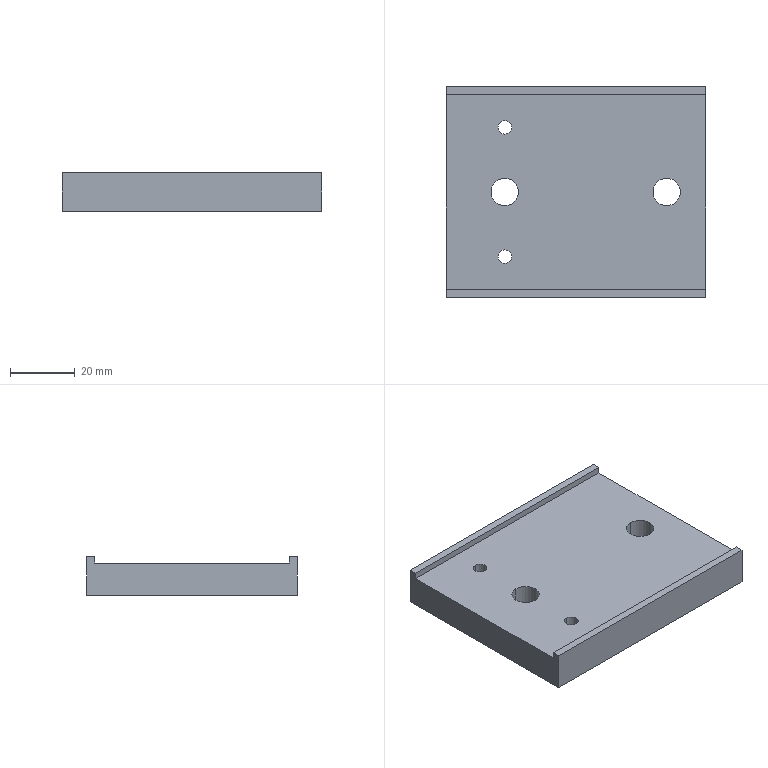Part | NX | 1 solid | 26 faces | box 80 x 65 x 12 mm | volume 50779 mm3 | cylinder 12 | plane 10 | cone 4 | commonest cylinder face diameters 4.2 x4 5 x4 8.5 x4
STEP:
#1=CARTESIAN_POINT('',(-22.,-17.9,-12.));
#2=VERTEX_POINT('',#1);
#3=CARTESIAN_POINT('',(-22.,-22.1,-12.));
#4=VERTEX_POINT('',#3);
#5=CARTESIAN_POINT('',(-22.,-20.,-12.));
#6=DIRECTION('',(0.,0.,1.));
#7=DIRECTION('',(0.,-1.,0.));
#8=AXIS2_PLACEMENT_3D('',#5,#6,#7);
#9=CIRCLE('',#8,2.1);
#10=EDGE_CURVE('',#2,#4,#9,.T.);
#11=ORIENTED_EDGE('',*,*,#10,.F.);
#12=CARTESIAN_POINT('',(-22.,-17.9,-2.));
#13=VERTEX_POINT('',#12);
#14=CARTESIAN_POINT('',(-22.,-17.9,-2.));
#15=DIRECTION('',(0.,0.,1.));
#16=VECTOR('',#15,1000.);
#17=LINE('',#14,#16);
#18=EDGE_CURVE('',#13,#2,#17,.F.);
#19=ORIENTED_EDGE('',*,*,#18,.F.);
#20=CARTESIAN_POINT('',(-22.,-22.1,-2.));
#21=VERTEX_POINT('',#20);
#22=CARTESIAN_POINT('',(-22.,-20.,-2.));
#23=DIRECTION('',(0.,0.,1.));
#24=DIRECTION('',(0.,-1.,0.));
#25=AXIS2_PLACEMENT_3D('',#22,#23,#24);
#26=CIRCLE('',#25,2.1);
#27=EDGE_CURVE('',#13,#21,#26,.T.);
#28=ORIENTED_EDGE('',*,*,#27,.T.);
#29=CARTESIAN_POINT('',(-22.,-22.1,-2.));
#30=DIRECTION('',(0.,0.,1.));
#31=VECTOR('',#30,1000.);
#32=LINE('',#29,#31);
#33=EDGE_CURVE('',#21,#4,#32,.F.);
#34=ORIENTED_EDGE('',*,*,#33,.T.);
#35=EDGE_LOOP('',(#11,#19,#28,#34));
#36=FACE_BOUND('',#35,.T.);
#37=CARTESIAN_POINT('',(-22.,-20.,-2.));
#38=DIRECTION('',(0.,0.,1.));
#39=DIRECTION('',(0.,1.,0.));
#40=AXIS2_PLACEMENT_3D('',#37,#38,#39);
#41=CYLINDRICAL_SURFACE('',#40,2.1);
#42=ADVANCED_FACE('',(#36),#41,.F.);
#43=CARTESIAN_POINT('',(-22.,22.1,-12.));
#44=VERTEX_POINT('',#43);
#45=CARTESIAN_POINT('',(-22.,17.9,-12.));
#46=VERTEX_POINT('',#45);
#47=CARTESIAN_POINT('',(-22.,20.,-12.));
#48=DIRECTION('',(0.,0.,1.));
#49=DIRECTION('',(0.,-1.,0.));
#50=AXIS2_PLACEMENT_3D('',#47,#48,#49);
#51=CIRCLE('',#50,2.1);
#52=EDGE_CURVE('',#44,#46,#51,.T.);
#53=ORIENTED_EDGE('',*,*,#52,.F.);
#54=CARTESIAN_POINT('',(-22.,22.1,-2.));
#55=VERTEX_POINT('',#54);
#56=CARTESIAN_POINT('',(-22.,22.1,-2.));
#57=DIRECTION('',(0.,0.,1.));
#58=VECTOR('',#57,1000.);
#59=LINE('',#56,#58);
#60=EDGE_CURVE('',#55,#44,#59,.F.);
#61=ORIENTED_EDGE('',*,*,#60,.F.);
#62=CARTESIAN_POINT('',(-22.,17.9,-2.));
#63=VERTEX_POINT('',#62);
#64=CARTESIAN_POINT('',(-22.,20.,-2.));
#65=DIRECTION('',(0.,0.,1.));
#66=DIRECTION('',(0.,-1.,0.));
#67=AXIS2_PLACEMENT_3D('',#64,#65,#66);
#68=CIRCLE('',#67,2.1);
#69=EDGE_CURVE('',#55,#63,#68,.T.);
#70=ORIENTED_EDGE('',*,*,#69,.T.);
#71=CARTESIAN_POINT('',(-22.,17.9,-2.));
#72=DIRECTION('',(0.,0.,1.));
#73=VECTOR('',#72,1000.);
#74=LINE('',#71,#73);
#75=EDGE_CURVE('',#63,#46,#74,.F.);
#76=ORIENTED_EDGE('',*,*,#75,.T.);
#77=EDGE_LOOP('',(#53,#61,#70,#76));
#78=FACE_BOUND('',#77,.T.);
#79=CARTESIAN_POINT('',(-22.,20.,-2.));
#80=DIRECTION('',(0.,0.,1.));
#81=DIRECTION('',(0.,1.,0.));
#82=AXIS2_PLACEMENT_3D('',#79,#80,#81);
#83=CYLINDRICAL_SURFACE('',#82,2.1);
#84=ADVANCED_FACE('',(#78),#83,.F.);
#85=CARTESIAN_POINT('',(25.,-22.5,-6.));
#86=VERTEX_POINT('',#85);
#87=CARTESIAN_POINT('',(25.,-17.5,-6.));
#88=VERTEX_POINT('',#87);
#89=CARTESIAN_POINT('',(25.,-20.,-6.));
#90=DIRECTION('',(1.,0.,0.));
#91=DIRECTION('',(0.,1.,0.));
#92=AXIS2_PLACEMENT_3D('',#89,#90,#91);
#93=CIRCLE('',#92,2.5);
#94=EDGE_CURVE('',#86,#88,#93,.T.);
#95=ORIENTED_EDGE('',*,*,#94,.F.);
#96=CARTESIAN_POINT('',(40.,-22.5,-6.));
#97=VERTEX_POINT('',#96);
#98=CARTESIAN_POINT('',(40.,-22.5,-6.));
#99=DIRECTION('',(1.,0.,0.));
#100=VECTOR('',#99,1000.);
#101=LINE('',#98,#100);
#102=EDGE_CURVE('',#97,#86,#101,.F.);
#103=ORIENTED_EDGE('',*,*,#102,.F.);
#104=CARTESIAN_POINT('',(40.,-17.5,-6.));
#105=VERTEX_POINT('',#104);
#106=CARTESIAN_POINT('',(40.,-20.,-6.));
#107=DIRECTION('',(1.,0.,0.));
#108=DIRECTION('',(0.,1.,0.));
#109=AXIS2_PLACEMENT_3D('',#106,#107,#108);
#110=CIRCLE('',#109,2.5);
#111=EDGE_CURVE('',#97,#105,#110,.T.);
#112=ORIENTED_EDGE('',*,*,#111,.T.);
#113=CARTESIAN_POINT('',(40.,-17.5,-6.));
#114=DIRECTION('',(1.,0.,0.));
#115=VECTOR('',#114,1000.);
#116=LINE('',#113,#115);
#117=EDGE_CURVE('',#105,#88,#116,.F.);
#118=ORIENTED_EDGE('',*,*,#117,.T.);
#119=EDGE_LOOP('',(#95,#103,#112,#118));
#120=FACE_BOUND('',#119,.T.);
#121=CARTESIAN_POINT('',(40.,-20.,-6.));
#122=DIRECTION('',(1.,0.,0.));
#123=DIRECTION('',(0.,-1.,0.));
#124=AXIS2_PLACEMENT_3D('',#121,#122,#123);
#125=CYLINDRICAL_SURFACE('',#124,2.5);
#126=ADVANCED_FACE('',(#120),#125,.F.);
#127=CARTESIAN_POINT('',(23.498,-20.,-6.));
#128=VERTEX_POINT('',#127);
#129=CARTESIAN_POINT('',(25.,-17.5,-6.));
#130=DIRECTION('',(0.515,0.8572,0.));
#131=VECTOR('',#130,1000.);
#132=LINE('',#129,#131);
#133=EDGE_CURVE('',#88,#128,#132,.F.);
#134=ORIENTED_EDGE('',*,*,#133,.T.);
#135=CARTESIAN_POINT('',(25.,-22.5,-6.));
#136=DIRECTION('',(0.515,-0.8572,0.));
#137=VECTOR('',#136,1000.);
#138=LINE('',#135,#137);
#139=EDGE_CURVE('',#86,#128,#138,.F.);
#140=ORIENTED_EDGE('',*,*,#139,.F.);
#141=ORIENTED_EDGE('',*,*,#94,.T.);
#142=EDGE_LOOP('',(#134,#140,#141));
#143=FACE_BOUND('',#142,.T.);
#144=CARTESIAN_POINT('',(25.,-20.,-6.));
#145=DIRECTION('',(1.,0.,0.));
#146=DIRECTION('',(0.,-1.,0.));
#147=AXIS2_PLACEMENT_3D('',#144,#145,#146);
#148=CONICAL_SURFACE('',#147,2.5,1.03);
#149=ADVANCED_FACE('',(#143),#148,.F.);
#150=CARTESIAN_POINT('',(25.,17.5,-6.));
#151=VERTEX_POINT('',#150);
#152=CARTESIAN_POINT('',(25.,22.5,-6.));
#153=VERTEX_POINT('',#152);
#154=CARTESIAN_POINT('',(25.,20.,-6.));
#155=DIRECTION('',(1.,0.,0.));
#156=DIRECTION('',(0.,1.,0.));
#157=AXIS2_PLACEMENT_3D('',#154,#155,#156);
#158=CIRCLE('',#157,2.5);
#159=EDGE_CURVE('',#151,#153,#158,.T.);
#160=ORIENTED_EDGE('',*,*,#159,.F.);
#161=CARTESIAN_POINT('',(40.,17.5,-6.));
#162=VERTEX_POINT('',#161);
#163=CARTESIAN_POINT('',(40.,17.5,-6.));
#164=DIRECTION('',(1.,0.,0.));
#165=VECTOR('',#164,1000.);
#166=LINE('',#163,#165);
#167=EDGE_CURVE('',#162,#151,#166,.F.);
#168=ORIENTED_EDGE('',*,*,#167,.F.);
#169=CARTESIAN_POINT('',(40.,22.5,-6.));
#170=VERTEX_POINT('',#169);
#171=CARTESIAN_POINT('',(40.,20.,-6.));
#172=DIRECTION('',(1.,0.,0.));
#173=DIRECTION('',(0.,1.,0.));
#174=AXIS2_PLACEMENT_3D('',#171,#172,#173);
#175=CIRCLE('',#174,2.5);
#176=EDGE_CURVE('',#162,#170,#175,.T.);
#177=ORIENTED_EDGE('',*,*,#176,.T.);
#178=CARTESIAN_POINT('',(40.,22.5,-6.));
#179=DIRECTION('',(1.,0.,0.));
#180=VECTOR('',#179,1000.);
#181=LINE('',#178,#180);
#182=EDGE_CURVE('',#170,#153,#181,.F.);
#183=ORIENTED_EDGE('',*,*,#182,.T.);
#184=EDGE_LOOP('',(#160,#168,#177,#183));
#185=FACE_BOUND('',#184,.T.);
#186=CARTESIAN_POINT('',(40.,20.,-6.));
#187=DIRECTION('',(1.,0.,0.));
#188=DIRECTION('',(0.,-1.,0.));
#189=AXIS2_PLACEMENT_3D('',#186,#187,#188);
#190=CYLINDRICAL_SURFACE('',#189,2.5);
#191=ADVANCED_FACE('',(#185),#190,.F.);
#192=CARTESIAN_POINT('',(23.498,20.,-6.));
#193=VERTEX_POINT('',#192);
#194=CARTESIAN_POINT('',(25.,22.5,-6.));
#195=DIRECTION('',(0.515,0.8572,0.));
#196=VECTOR('',#195,1000.);
#197=LINE('',#194,#196);
#198=EDGE_CURVE('',#153,#193,#197,.F.);
#199=ORIENTED_EDGE('',*,*,#198,.T.);
#200=CARTESIAN_POINT('',(25.,17.5,-6.));
#201=DIRECTION('',(0.515,-0.8572,0.));
#202=VECTOR('',#201,1000.);
#203=LINE('',#200,#202);
#204=EDGE_CURVE('',#151,#193,#203,.F.);
#205=ORIENTED_EDGE('',*,*,#204,.F.);
#206=ORIENTED_EDGE('',*,*,#159,.T.);
#207=EDGE_LOOP('',(#199,#205,#206));
#208=FACE_BOUND('',#207,.T.);
#209=CARTESIAN_POINT('',(25.,20.,-6.));
#210=DIRECTION('',(1.,0.,0.));
#211=DIRECTION('',(0.,-1.,0.));
#212=AXIS2_PLACEMENT_3D('',#209,#210,#211);
#213=CONICAL_SURFACE('',#212,2.5,1.03);
#214=ADVANCED_FACE('',(#208),#213,.F.);
#215=CARTESIAN_POINT('',(28.,4.25,-12.));
#216=VERTEX_POINT('',#215);
#217=CARTESIAN_POINT('',(28.,-4.25,-12.));
#218=VERTEX_POINT('',#217);
#219=CARTESIAN_POINT('',(28.,0.,-12.));
#220=DIRECTION('',(0.,0.,1.));
#221=DIRECTION('',(0.,-1.,0.));
#222=AXIS2_PLACEMENT_3D('',#219,#220,#221);
#223=CIRCLE('',#222,4.25);
#224=EDGE_CURVE('',#216,#218,#223,.T.);
#225=ORIENTED_EDGE('',*,*,#224,.F.);
#226=CARTESIAN_POINT('',(28.,4.25,-2.));
#227=VERTEX_POINT('',#226);
#228=CARTESIAN_POINT('',(28.,4.25,-2.));
#229=DIRECTION('',(0.,0.,1.));
#230=VECTOR('',#229,1000.);
#231=LINE('',#228,#230);
#232=EDGE_CURVE('',#227,#216,#231,.F.);
#233=ORIENTED_EDGE('',*,*,#232,.F.);
#234=CARTESIAN_POINT('',(28.,-4.25,-2.));
#235=VERTEX_POINT('',#234);
#236=CARTESIAN_POINT('',(28.,0.,-2.));
#237=DIRECTION('',(0.,0.,1.));
#238=DIRECTION('',(0.,-1.,0.));
#239=AXIS2_PLACEMENT_3D('',#236,#237,#238);
#240=CIRCLE('',#239,4.25);
#241=EDGE_CURVE('',#227,#235,#240,.T.);
#242=ORIENTED_EDGE('',*,*,#241,.T.);
#243=CARTESIAN_POINT('',(28.,-4.25,-2.));
#244=DIRECTION('',(0.,0.,1.));
#245=VECTOR('',#244,1000.);
#246=LINE('',#243,#245);
#247=EDGE_CURVE('',#235,#218,#246,.F.);
#248=ORIENTED_EDGE('',*,*,#247,.T.);
#249=EDGE_LOOP('',(#225,#233,#242,#248));
#250=FACE_BOUND('',#249,.T.);
#251=CARTESIAN_POINT('',(28.,0.,-2.));
#252=DIRECTION('',(0.,0.,1.));
#253=DIRECTION('',(0.,1.,0.));
#254=AXIS2_PLACEMENT_3D('',#251,#252,#253);
#255=CYLINDRICAL_SURFACE('',#254,4.25);
#256=ADVANCED_FACE('',(#250),#255,.F.);
#257=CARTESIAN_POINT('',(-22.,4.25,-12.));
#258=VERTEX_POINT('',#257);
#259=CARTESIAN_POINT('',(-22.,-4.25,-12.));
#260=VERTEX_POINT('',#259);
#261=CARTESIAN_POINT('',(-22.,0.,-12.));
#262=DIRECTION('',(0.,0.,1.));
#263=DIRECTION('',(0.,-1.,0.));
#264=AXIS2_PLACEMENT_3D('',#261,#262,#263);
#265=CIRCLE('',#264,4.25);
#266=EDGE_CURVE('',#258,#260,#265,.T.);
#267=ORIENTED_EDGE('',*,*,#266,.F.);
#268=CARTESIAN_POINT('',(-22.,4.25,-2.));
#269=VERTEX_POINT('',#268);
#270=CARTESIAN_POINT('',(-22.,4.25,-2.));
#271=DIRECTION('',(0.,0.,1.));
#272=VECTOR('',#271,1000.);
#273=LINE('',#270,#272);
#274=EDGE_CURVE('',#269,#258,#273,.F.);
#275=ORIENTED_EDGE('',*,*,#274,.F.);
#276=CARTESIAN_POINT('',(-22.,-4.25,-2.));
#277=VERTEX_POINT('',#276);
#278=CARTESIAN_POINT('',(-22.,0.,-2.));
#279=DIRECTION('',(0.,0.,1.));
#280=DIRECTION('',(0.,-1.,0.));
#281=AXIS2_PLACEMENT_3D('',#278,#279,#280);
#282=CIRCLE('',#281,4.25);
#283=EDGE_CURVE('',#269,#277,#282,.T.);
#284=ORIENTED_EDGE('',*,*,#283,.T.);
#285=CARTESIAN_POINT('',(-22.,-4.25,-2.));
#286=DIRECTION('',(0.,0.,1.));
#287=VECTOR('',#286,1000.);
#288=LINE('',#285,#287);
#289=EDGE_CURVE('',#277,#260,#288,.F.);
#290=ORIENTED_EDGE('',*,*,#289,.T.);
#291=EDGE_LOOP('',(#267,#275,#284,#290));
#292=FACE_BOUND('',#291,.T.);
#293=CARTESIAN_POINT('',(-22.,0.,-2.));
#294=DIRECTION('',(0.,0.,1.));
#295=DIRECTION('',(0.,1.,0.));
#296=AXIS2_PLACEMENT_3D('',#293,#294,#295);
#297=CYLINDRICAL_SURFACE('',#296,4.25);
#298=ADVANCED_FACE('',(#292),#297,.F.);
#299=CARTESIAN_POINT('',(40.,-32.5,0.));
#300=VERTEX_POINT('',#299);
#301=CARTESIAN_POINT('',(-40.,-32.5,0.));
#302=VERTEX_POINT('',#301);
#303=CARTESIAN_POINT('',(-40.,-32.5,0.));
#304=DIRECTION('',(-1.,0.,0.));
#305=VECTOR('',#304,1000.);
#306=LINE('',#303,#305);
#307=EDGE_CURVE('',#300,#302,#306,.T.);
#308=ORIENTED_EDGE('',*,*,#307,.F.);
#309=CARTESIAN_POINT('',(40.,-30.,0.));
#310=VERTEX_POINT('',#309);
#311=CARTESIAN_POINT('',(40.,-35.,0.));
#312=DIRECTION('',(0.,1.,0.));
#313=VECTOR('',#312,1000.);
#314=LINE('',#311,#313);
#315=EDGE_CURVE('',#300,#310,#314,.T.);
#316=ORIENTED_EDGE('',*,*,#315,.T.);
#317=CARTESIAN_POINT('',(-40.,-30.,0.));
#318=VERTEX_POINT('',#317);
#319=CARTESIAN_POINT('',(-40.,-30.,0.));
#320=DIRECTION('',(1.,0.,0.));
#321=VECTOR('',#320,1000.);
#322=LINE('',#319,#321);
#323=EDGE_CURVE('',#318,#310,#322,.T.);
#324=ORIENTED_EDGE('',*,*,#323,.F.);
#325=CARTESIAN_POINT('',(-40.,-35.,0.));
#326=DIRECTION('',(0.,1.,0.));
#327=VECTOR('',#326,1000.);
#328=LINE('',#325,#327);
#329=EDGE_CURVE('',#302,#318,#328,.T.);
#330=ORIENTED_EDGE('',*,*,#329,.F.);
#331=EDGE_LOOP('',(#308,#316,#324,#330));
#332=FACE_BOUND('',#331,.T.);
#333=CARTESIAN_POINT('',(-40.,-35.,0.));
#334=DIRECTION('',(0.,0.,-1.));
#335=DIRECTION('',(0.,-1.,0.));
#336=AXIS2_PLACEMENT_3D('',#333,#334,#335);
#337=PLANE('',#336);
#338=ADVANCED_FACE('',(#332),#337,.F.);
#339=CARTESIAN_POINT('',(40.,20.,-6.));
#340=DIRECTION('',(1.,0.,0.));
#341=DIRECTION('',(0.,1.,0.));
#342=AXIS2_PLACEMENT_3D('',#339,#340,#341);
#343=CIRCLE('',#342,2.5);
#344=EDGE_CURVE('',#170,#162,#343,.T.);
#345=ORIENTED_EDGE('',*,*,#344,.F.);
#346=ORIENTED_EDGE('',*,*,#176,.F.);
#347=EDGE_LOOP('',(#345,#346));
#348=FACE_BOUND('',#347,.T.);
#349=CARTESIAN_POINT('',(40.,-20.,-6.));
#350=DIRECTION('',(1.,0.,0.));
#351=DIRECTION('',(0.,1.,0.));
#352=AXIS2_PLACEMENT_3D('',#349,#350,#351);
#353=CIRCLE('',#352,2.5);
#354=EDGE_CURVE('',#105,#97,#353,.T.);
#355=ORIENTED_EDGE('',*,*,#354,.F.);
#356=ORIENTED_EDGE('',*,*,#111,.F.);
#357=EDGE_LOOP('',(#355,#356));
#358=FACE_BOUND('',#357,.T.);
#359=CARTESIAN_POINT('',(40.,-32.5,-12.));
#360=VERTEX_POINT('',#359);
#361=CARTESIAN_POINT('',(40.,-32.5,-12.));
#362=DIRECTION('',(0.,0.,1.));
#363=VECTOR('',#362,1000.);
#364=LINE('',#361,#363);
#365=EDGE_CURVE('',#360,#300,#364,.T.);
#366=ORIENTED_EDGE('',*,*,#365,.F.);
#367=CARTESIAN_POINT('',(40.,32.5,-12.));
#368=VERTEX_POINT('',#367);
#369=CARTESIAN_POINT('',(40.,-35.,-12.));
#370=DIRECTION('',(0.,1.,0.));
#371=VECTOR('',#370,1000.);
#372=LINE('',#369,#371);
#373=EDGE_CURVE('',#360,#368,#372,.T.);
#374=ORIENTED_EDGE('',*,*,#373,.T.);
#375=CARTESIAN_POINT('',(40.,32.5,0.));
#376=VERTEX_POINT('',#375);
#377=CARTESIAN_POINT('',(40.,32.5,-12.));
#378=DIRECTION('',(0.,0.,1.));
#379=VECTOR('',#378,1000.);
#380=LINE('',#377,#379);
#381=EDGE_CURVE('',#368,#376,#380,.T.);
#382=ORIENTED_EDGE('',*,*,#381,.T.);
#383=CARTESIAN_POINT('',(40.,30.,0.));
#384=VERTEX_POINT('',#383);
#385=CARTESIAN_POINT('',(40.,-35.,0.));
#386=DIRECTION('',(0.,1.,0.));
#387=VECTOR('',#386,1000.);
#388=LINE('',#385,#387);
#389=EDGE_CURVE('',#384,#376,#388,.T.);
#390=ORIENTED_EDGE('',*,*,#389,.F.);
#391=CARTESIAN_POINT('',(40.,30.,-2.));
#392=VERTEX_POINT('',#391);
#393=CARTESIAN_POINT('',(40.,30.,-2.));
#394=DIRECTION('',(0.,0.,1.));
#395=VECTOR('',#394,1000.);
#396=LINE('',#393,#395);
#397=EDGE_CURVE('',#392,#384,#396,.T.);
#398=ORIENTED_EDGE('',*,*,#397,.F.);
#399=CARTESIAN_POINT('',(40.,-30.,-2.));
#400=VERTEX_POINT('',#399);
#401=CARTESIAN_POINT('',(40.,30.,-2.));
#402=DIRECTION('',(0.,1.,0.));
#403=VECTOR('',#402,1000.);
#404=LINE('',#401,#403);
#405=EDGE_CURVE('',#400,#392,#404,.T.);
#406=ORIENTED_EDGE('',*,*,#405,.F.);
#407=CARTESIAN_POINT('',(40.,-30.,-2.));
#408=DIRECTION('',(0.,0.,1.));
#409=VECTOR('',#408,1000.);
#410=LINE('',#407,#409);
#411=EDGE_CURVE('',#400,#310,#410,.T.);
#412=ORIENTED_EDGE('',*,*,#411,.T.);
#413=ORIENTED_EDGE('',*,*,#315,.F.);
#414=EDGE_LOOP('',(#366,#374,#382,#390,#398,#406,#412,#413));
#415=FACE_BOUND('',#414,.T.);
#416=CARTESIAN_POINT('',(40.,-35.,-12.));
#417=DIRECTION('',(-1.,0.,0.));
#418=DIRECTION('',(0.,1.,0.));
#419=AXIS2_PLACEMENT_3D('',#416,#417,#418);
#420=PLANE('',#419);
#421=ADVANCED_FACE('',(#348,#358,#415),#420,.F.);
#422=CARTESIAN_POINT('',(-40.,-32.5,-12.));
#423=VERTEX_POINT('',#422);
#424=CARTESIAN_POINT('',(-40.,-32.5,-12.));
#425=DIRECTION('',(0.,0.,-1.));
#426=VECTOR('',#425,1000.);
#427=LINE('',#424,#426);
#428=EDGE_CURVE('',#302,#423,#427,.T.);
#429=ORIENTED_EDGE('',*,*,#428,.F.);
#430=ORIENTED_EDGE('',*,*,#329,.T.);
#431=CARTESIAN_POINT('',(-40.,-30.,-2.));
#432=VERTEX_POINT('',#431);
#433=CARTESIAN_POINT('',(-40.,-30.,-2.));
#434=DIRECTION('',(0.,0.,1.));
#435=VECTOR('',#434,1000.);
#436=LINE('',#433,#435);
#437=EDGE_CURVE('',#432,#318,#436,.T.);
#438=ORIENTED_EDGE('',*,*,#437,.F.);
#439=CARTESIAN_POINT('',(-40.,30.,-2.));
#440=VERTEX_POINT('',#439);
#441=CARTESIAN_POINT('',(-40.,30.,-2.));
#442=DIRECTION('',(0.,-1.,0.));
#443=VECTOR('',#442,1000.);
#444=LINE('',#441,#443);
#445=EDGE_CURVE('',#440,#432,#444,.T.);
#446=ORIENTED_EDGE('',*,*,#445,.F.);
#447=CARTESIAN_POINT('',(-40.,30.,0.));
#448=VERTEX_POINT('',#447);
#449=CARTESIAN_POINT('',(-40.,30.,-2.));
#450=DIRECTION('',(0.,0.,1.));
#451=VECTOR('',#450,1000.);
#452=LINE('',#449,#451);
#453=EDGE_CURVE('',#440,#448,#452,.T.);
#454=ORIENTED_EDGE('',*,*,#453,.T.);
#455=CARTESIAN_POINT('',(-40.,32.5,0.));
#456=VERTEX_POINT('',#455);
#457=CARTESIAN_POINT('',(-40.,-35.,0.));
#458=DIRECTION('',(0.,1.,0.));
#459=VECTOR('',#458,1000.);
#460=LINE('',#457,#459);
#461=EDGE_CURVE('',#448,#456,#460,.T.);
#462=ORIENTED_EDGE('',*,*,#461,.T.);
#463=CARTESIAN_POINT('',(-40.,32.5,-12.));
#464=VERTEX_POINT('',#463);
#465=CARTESIAN_POINT('',(-40.,32.5,-12.));
#466=DIRECTION('',(0.,0.,-1.));
#467=VECTOR('',#466,1000.);
#468=LINE('',#465,#467);
#469=EDGE_CURVE('',#456,#464,#468,.T.);
#470=ORIENTED_EDGE('',*,*,#469,.T.);
#471=CARTESIAN_POINT('',(-40.,-35.,-12.));
#472=DIRECTION('',(0.,1.,0.));
#473=VECTOR('',#472,1000.);
#474=LINE('',#471,#473);
#475=EDGE_CURVE('',#423,#464,#474,.T.);
#476=ORIENTED_EDGE('',*,*,#475,.F.);
#477=EDGE_LOOP('',(#429,#430,#438,#446,#454,#462,#470,#476));
#478=FACE_BOUND('',#477,.T.);
#479=CARTESIAN_POINT('',(-40.,-35.,-12.));
#480=DIRECTION('',(1.,0.,0.));
#481=DIRECTION('',(0.,-1.,0.));
#482=AXIS2_PLACEMENT_3D('',#479,#480,#481);
#483=PLANE('',#482);
#484=ADVANCED_FACE('',(#478),#483,.F.);
#485=CARTESIAN_POINT('',(-22.,-20.,-12.));
#486=DIRECTION('',(0.,0.,1.));
#487=DIRECTION('',(0.,-1.,0.));
#488=AXIS2_PLACEMENT_3D('',#485,#486,#487);
#489=CIRCLE('',#488,2.1);
#490=EDGE_CURVE('',#4,#2,#489,.T.);
#491=ORIENTED_EDGE('',*,*,#490,.T.);
#492=ORIENTED_EDGE('',*,*,#10,.T.);
#493=EDGE_LOOP('',(#491,#492));
#494=FACE_BOUND('',#493,.T.);
#495=CARTESIAN_POINT('',(-22.,20.,-12.));
#496=DIRECTION('',(0.,0.,1.));
#497=DIRECTION('',(0.,-1.,0.));
#498=AXIS2_PLACEMENT_3D('',#495,#496,#497);
#499=CIRCLE('',#498,2.1);
#500=EDGE_CURVE('',#46,#44,#499,.T.);
#501=ORIENTED_EDGE('',*,*,#500,.T.);
#502=ORIENTED_EDGE('',*,*,#52,.T.);
#503=EDGE_LOOP('',(#501,#502));
#504=FACE_BOUND('',#503,.T.);
#505=CARTESIAN_POINT('',(-22.,0.,-12.));
#506=DIRECTION('',(0.,0.,1.));
#507=DIRECTION('',(0.,-1.,0.));
#508=AXIS2_PLACEMENT_3D('',#505,#506,#507);
#509=CIRCLE('',#508,4.25);
#510=EDGE_CURVE('',#260,#258,#509,.T.);
#511=ORIENTED_EDGE('',*,*,#510,.T.);
#512=ORIENTED_EDGE('',*,*,#266,.T.);
#513=EDGE_LOOP('',(#511,#512));
#514=FACE_BOUND('',#513,.T.);
#515=CARTESIAN_POINT('',(28.,0.,-12.));
#516=DIRECTION('',(0.,0.,1.));
#517=DIRECTION('',(0.,-1.,0.));
#518=AXIS2_PLACEMENT_3D('',#515,#516,#517);
#519=CIRCLE('',#518,4.25);
#520=EDGE_CURVE('',#218,#216,#519,.T.);
#521=ORIENTED_EDGE('',*,*,#520,.T.);
#522=ORIENTED_EDGE('',*,*,#224,.T.);
#523=EDGE_LOOP('',(#521,#522));
#524=FACE_BOUND('',#523,.T.);
#525=CARTESIAN_POINT('',(-40.,-32.5,-12.));
#526=DIRECTION('',(1.,0.,0.));
#527=VECTOR('',#526,1000.);
#528=LINE('',#525,#527);
#529=EDGE_CURVE('',#423,#360,#528,.T.);
#530=ORIENTED_EDGE('',*,*,#529,.F.);
#531=ORIENTED_EDGE('',*,*,#475,.T.);
#532=CARTESIAN_POINT('',(-40.,32.5,-12.));
#533=DIRECTION('',(1.,0.,0.));
#534=VECTOR('',#533,1000.);
#535=LINE('',#532,#534);
#536=EDGE_CURVE('',#464,#368,#535,.T.);
#537=ORIENTED_EDGE('',*,*,#536,.T.);
#538=ORIENTED_EDGE('',*,*,#373,.F.);
#539=EDGE_LOOP('',(#530,#531,#537,#538));
#540=FACE_BOUND('',#539,.T.);
#541=CARTESIAN_POINT('',(-40.,-35.,-12.));
#542=DIRECTION('',(0.,0.,1.));
#543=DIRECTION('',(0.,1.,0.));
#544=AXIS2_PLACEMENT_3D('',#541,#542,#543);
#545=PLANE('',#544);
#546=ADVANCED_FACE('',(#494,#504,#514,#524,#540),#545,.F.);
#547=ORIENTED_EDGE('',*,*,#389,.T.);
#548=CARTESIAN_POINT('',(-40.,32.5,0.));
#549=DIRECTION('',(-1.,0.,0.));
#550=VECTOR('',#549,1000.);
#551=LINE('',#548,#550);
#552=EDGE_CURVE('',#376,#456,#551,.T.);
#553=ORIENTED_EDGE('',*,*,#552,.T.);
#554=ORIENTED_EDGE('',*,*,#461,.F.);
#555=CARTESIAN_POINT('',(-40.,30.,0.));
#556=DIRECTION('',(-1.,0.,0.));
#557=VECTOR('',#556,1000.);
#558=LINE('',#555,#557);
#559=EDGE_CURVE('',#384,#448,#558,.T.);
#560=ORIENTED_EDGE('',*,*,#559,.F.);
#561=EDGE_LOOP('',(#547,#553,#554,#560));
#562=FACE_BOUND('',#561,.T.);
#563=CARTESIAN_POINT('',(-40.,-35.,0.));
#564=DIRECTION('',(0.,0.,-1.));
#565=DIRECTION('',(0.,-1.,0.));
#566=AXIS2_PLACEMENT_3D('',#563,#564,#565);
#567=PLANE('',#566);
#568=ADVANCED_FACE('',(#562),#567,.F.);
#569=ORIENTED_EDGE('',*,*,#323,.T.);
#570=ORIENTED_EDGE('',*,*,#411,.F.);
#571=CARTESIAN_POINT('',(-40.,-30.,-2.));
#572=DIRECTION('',(1.,0.,0.));
#573=VECTOR('',#572,1000.);
#574=LINE('',#571,#573);
#575=EDGE_CURVE('',#432,#400,#574,.T.);
#576=ORIENTED_EDGE('',*,*,#575,.F.);
#577=ORIENTED_EDGE('',*,*,#437,.T.);
#578=EDGE_LOOP('',(#569,#570,#576,#577));
#579=FACE_BOUND('',#578,.T.);
#580=CARTESIAN_POINT('',(-40.,-30.,-2.));
#581=DIRECTION('',(0.,-1.,0.));
#582=DIRECTION('',(-1.,0.,0.));
#583=AXIS2_PLACEMENT_3D('',#580,#581,#582);
#584=PLANE('',#583);
#585=ADVANCED_FACE('',(#579),#584,.F.);
#586=ORIENTED_EDGE('',*,*,#559,.T.);
#587=ORIENTED_EDGE('',*,*,#453,.F.);
#588=CARTESIAN_POINT('',(-40.,30.,-2.));
#589=DIRECTION('',(-1.,0.,0.));
#590=VECTOR('',#589,1000.);
#591=LINE('',#588,#590);
#592=EDGE_CURVE('',#392,#440,#591,.T.);
#593=ORIENTED_EDGE('',*,*,#592,.F.);
#594=ORIENTED_EDGE('',*,*,#397,.T.);
#595=EDGE_LOOP('',(#586,#587,#593,#594));
#596=FACE_BOUND('',#595,.T.);
#597=CARTESIAN_POINT('',(-40.,30.,-2.));
#598=DIRECTION('',(0.,1.,0.));
#599=DIRECTION('',(1.,0.,0.));
#600=AXIS2_PLACEMENT_3D('',#597,#598,#599);
#601=PLANE('',#600);
#602=ADVANCED_FACE('',(#596),#601,.F.);
#603=CARTESIAN_POINT('',(-22.,-20.,-2.));
#604=DIRECTION('',(0.,0.,1.));
#605=DIRECTION('',(0.,-1.,0.));
#606=AXIS2_PLACEMENT_3D('',#603,#604,#605);
#607=CIRCLE('',#606,2.1);
#608=EDGE_CURVE('',#21,#13,#607,.T.);
#609=ORIENTED_EDGE('',*,*,#608,.F.);
#610=ORIENTED_EDGE('',*,*,#27,.F.);
#611=EDGE_LOOP('',(#609,#610));
#612=FACE_BOUND('',#611,.T.);
#613=CARTESIAN_POINT('',(-22.,20.,-2.));
#614=DIRECTION('',(0.,0.,1.));
#615=DIRECTION('',(0.,-1.,0.));
#616=AXIS2_PLACEMENT_3D('',#613,#614,#615);
#617=CIRCLE('',#616,2.1);
#618=EDGE_CURVE('',#63,#55,#617,.T.);
#619=ORIENTED_EDGE('',*,*,#618,.F.);
#620=ORIENTED_EDGE('',*,*,#69,.F.);
#621=EDGE_LOOP('',(#619,#620));
#622=FACE_BOUND('',#621,.T.);
#623=CARTESIAN_POINT('',(28.,0.,-2.));
#624=DIRECTION('',(0.,0.,1.));
#625=DIRECTION('',(0.,-1.,0.));
#626=AXIS2_PLACEMENT_3D('',#623,#624,#625);
#627=CIRCLE('',#626,4.25);
#628=EDGE_CURVE('',#235,#227,#627,.T.);
#629=ORIENTED_EDGE('',*,*,#628,.F.);
#630=ORIENTED_EDGE('',*,*,#241,.F.);
#631=EDGE_LOOP('',(#629,#630));
#632=FACE_BOUND('',#631,.T.);
#633=CARTESIAN_POINT('',(-22.,0.,-2.));
#634=DIRECTION('',(0.,0.,1.));
#635=DIRECTION('',(0.,-1.,0.));
#636=AXIS2_PLACEMENT_3D('',#633,#634,#635);
#637=CIRCLE('',#636,4.25);
#638=EDGE_CURVE('',#277,#269,#637,.T.);
#639=ORIENTED_EDGE('',*,*,#638,.F.);
#640=ORIENTED_EDGE('',*,*,#283,.F.);
#641=EDGE_LOOP('',(#639,#640));
#642=FACE_BOUND('',#641,.T.);
#643=ORIENTED_EDGE('',*,*,#405,.T.);
#644=ORIENTED_EDGE('',*,*,#592,.T.);
#645=ORIENTED_EDGE('',*,*,#445,.T.);
#646=ORIENTED_EDGE('',*,*,#575,.T.);
#647=EDGE_LOOP('',(#643,#644,#645,#646));
#648=FACE_BOUND('',#647,.T.);
#649=CARTESIAN_POINT('',(0.,35.,-2.));
#650=DIRECTION('',(0.,0.,1.));
#651=DIRECTION('',(0.,1.,0.));
#652=AXIS2_PLACEMENT_3D('',#649,#650,#651);
#653=PLANE('',#652);
#654=ADVANCED_FACE('',(#612,#622,#632,#642,#648),#653,.T.);
#655=ORIENTED_EDGE('',*,*,#274,.T.);
#656=ORIENTED_EDGE('',*,*,#510,.F.);
#657=ORIENTED_EDGE('',*,*,#289,.F.);
#658=ORIENTED_EDGE('',*,*,#638,.T.);
#659=EDGE_LOOP('',(#655,#656,#657,#658));
#660=FACE_BOUND('',#659,.T.);
#661=CARTESIAN_POINT('',(-22.,0.,-2.));
#662=DIRECTION('',(0.,0.,1.));
#663=DIRECTION('',(0.,1.,0.));
#664=AXIS2_PLACEMENT_3D('',#661,#662,#663);
#665=CYLINDRICAL_SURFACE('',#664,4.25);
#666=ADVANCED_FACE('',(#660),#665,.F.);
#667=ORIENTED_EDGE('',*,*,#232,.T.);
#668=ORIENTED_EDGE('',*,*,#520,.F.);
#669=ORIENTED_EDGE('',*,*,#247,.F.);
#670=ORIENTED_EDGE('',*,*,#628,.T.);
#671=EDGE_LOOP('',(#667,#668,#669,#670));
#672=FACE_BOUND('',#671,.T.);
#673=CARTESIAN_POINT('',(28.,0.,-2.));
#674=DIRECTION('',(0.,0.,1.));
#675=DIRECTION('',(0.,1.,0.));
#676=AXIS2_PLACEMENT_3D('',#673,#674,#675);
#677=CYLINDRICAL_SURFACE('',#676,4.25);
#678=ADVANCED_FACE('',(#672),#677,.F.);
#679=ORIENTED_EDGE('',*,*,#204,.T.);
#680=ORIENTED_EDGE('',*,*,#198,.F.);
#681=CARTESIAN_POINT('',(25.,20.,-6.));
#682=DIRECTION('',(1.,0.,0.));
#683=DIRECTION('',(0.,1.,0.));
#684=AXIS2_PLACEMENT_3D('',#681,#682,#683);
#685=CIRCLE('',#684,2.5);
#686=EDGE_CURVE('',#153,#151,#685,.T.);
#687=ORIENTED_EDGE('',*,*,#686,.T.);
#688=EDGE_LOOP('',(#679,#680,#687));
#689=FACE_BOUND('',#688,.T.);
#690=CARTESIAN_POINT('',(25.,20.,-6.));
#691=DIRECTION('',(1.,0.,0.));
#692=DIRECTION('',(0.,-1.,0.));
#693=AXIS2_PLACEMENT_3D('',#690,#691,#692);
#694=CONICAL_SURFACE('',#693,2.5,1.03);
#695=ADVANCED_FACE('',(#689),#694,.F.);
#696=ORIENTED_EDGE('',*,*,#167,.T.);
#697=ORIENTED_EDGE('',*,*,#686,.F.);
#698=ORIENTED_EDGE('',*,*,#182,.F.);
#699=ORIENTED_EDGE('',*,*,#344,.T.);
#700=EDGE_LOOP('',(#696,#697,#698,#699));
#701=FACE_BOUND('',#700,.T.);
#702=CARTESIAN_POINT('',(40.,20.,-6.));
#703=DIRECTION('',(1.,0.,0.));
#704=DIRECTION('',(0.,-1.,0.));
#705=AXIS2_PLACEMENT_3D('',#702,#703,#704);
#706=CYLINDRICAL_SURFACE('',#705,2.5);
#707=ADVANCED_FACE('',(#701),#706,.F.);
#708=ORIENTED_EDGE('',*,*,#139,.T.);
#709=ORIENTED_EDGE('',*,*,#133,.F.);
#710=CARTESIAN_POINT('',(25.,-20.,-6.));
#711=DIRECTION('',(1.,0.,0.));
#712=DIRECTION('',(0.,1.,0.));
#713=AXIS2_PLACEMENT_3D('',#710,#711,#712);
#714=CIRCLE('',#713,2.5);
#715=EDGE_CURVE('',#88,#86,#714,.T.);
#716=ORIENTED_EDGE('',*,*,#715,.T.);
#717=EDGE_LOOP('',(#708,#709,#716));
#718=FACE_BOUND('',#717,.T.);
#719=CARTESIAN_POINT('',(25.,-20.,-6.));
#720=DIRECTION('',(1.,0.,0.));
#721=DIRECTION('',(0.,-1.,0.));
#722=AXIS2_PLACEMENT_3D('',#719,#720,#721);
#723=CONICAL_SURFACE('',#722,2.5,1.03);
#724=ADVANCED_FACE('',(#718),#723,.F.);
#725=ORIENTED_EDGE('',*,*,#102,.T.);
#726=ORIENTED_EDGE('',*,*,#715,.F.);
#727=ORIENTED_EDGE('',*,*,#117,.F.);
#728=ORIENTED_EDGE('',*,*,#354,.T.);
#729=EDGE_LOOP('',(#725,#726,#727,#728));
#730=FACE_BOUND('',#729,.T.);
#731=CARTESIAN_POINT('',(40.,-20.,-6.));
#732=DIRECTION('',(1.,0.,0.));
#733=DIRECTION('',(0.,-1.,0.));
#734=AXIS2_PLACEMENT_3D('',#731,#732,#733);
#735=CYLINDRICAL_SURFACE('',#734,2.5);
#736=ADVANCED_FACE('',(#730),#735,.F.);
#737=ORIENTED_EDGE('',*,*,#536,.F.);
#738=ORIENTED_EDGE('',*,*,#469,.F.);
#739=ORIENTED_EDGE('',*,*,#552,.F.);
#740=ORIENTED_EDGE('',*,*,#381,.F.);
#741=EDGE_LOOP('',(#737,#738,#739,#740));
#742=FACE_BOUND('',#741,.T.);
#743=CARTESIAN_POINT('',(0.,32.5,-6.));
#744=DIRECTION('',(0.,-1.,0.));
#745=DIRECTION('',(-1.,0.,0.));
#746=AXIS2_PLACEMENT_3D('',#743,#744,#745);
#747=PLANE('',#746);
#748=ADVANCED_FACE('',(#742),#747,.F.);
#749=ORIENTED_EDGE('',*,*,#307,.T.);
#750=ORIENTED_EDGE('',*,*,#428,.T.);
#751=ORIENTED_EDGE('',*,*,#529,.T.);
#752=ORIENTED_EDGE('',*,*,#365,.T.);
#753=EDGE_LOOP('',(#749,#750,#751,#752));
#754=FACE_BOUND('',#753,.T.);
#755=CARTESIAN_POINT('',(0.,-32.5,-6.));
#756=DIRECTION('',(0.,-1.,0.));
#757=DIRECTION('',(-1.,0.,0.));
#758=AXIS2_PLACEMENT_3D('',#755,#756,#757);
#759=PLANE('',#758);
#760=ADVANCED_FACE('',(#754),#759,.T.);
#761=ORIENTED_EDGE('',*,*,#60,.T.);
#762=ORIENTED_EDGE('',*,*,#500,.F.);
#763=ORIENTED_EDGE('',*,*,#75,.F.);
#764=ORIENTED_EDGE('',*,*,#618,.T.);
#765=EDGE_LOOP('',(#761,#762,#763,#764));
#766=FACE_BOUND('',#765,.T.);
#767=CARTESIAN_POINT('',(-22.,20.,-2.));
#768=DIRECTION('',(0.,0.,1.));
#769=DIRECTION('',(0.,1.,0.));
#770=AXIS2_PLACEMENT_3D('',#767,#768,#769);
#771=CYLINDRICAL_SURFACE('',#770,2.1);
#772=ADVANCED_FACE('',(#766),#771,.F.);
#773=ORIENTED_EDGE('',*,*,#18,.T.);
#774=ORIENTED_EDGE('',*,*,#490,.F.);
#775=ORIENTED_EDGE('',*,*,#33,.F.);
#776=ORIENTED_EDGE('',*,*,#608,.T.);
#777=EDGE_LOOP('',(#773,#774,#775,#776));
#778=FACE_BOUND('',#777,.T.);
#779=CARTESIAN_POINT('',(-22.,-20.,-2.));
#780=DIRECTION('',(0.,0.,1.));
#781=DIRECTION('',(0.,1.,0.));
#782=AXIS2_PLACEMENT_3D('',#779,#780,#781);
#783=CYLINDRICAL_SURFACE('',#782,2.1);
#784=ADVANCED_FACE('',(#778),#783,.F.);
#785=CLOSED_SHELL('',(#42,#84,#126,#149,#191,#214,#256,#298,#338,#421,#484,#546,#568,#585,#602,#654,#666,#678,#695,#707,#724,#736,#748,#760,#772,#784));
#786=MANIFOLD_SOLID_BREP('',#785);
#787=(LENGTH_UNIT()NAMED_UNIT(*)SI_UNIT(.MILLI.,.METRE.));
#788=UNCERTAINTY_MEASURE_WITH_UNIT(LENGTH_MEASURE(0.00001),#787,'','');
#789=(NAMED_UNIT(*)PLANE_ANGLE_UNIT()SI_UNIT($,.RADIAN.));
#790=(NAMED_UNIT(*)SI_UNIT($,.STERADIAN.)SOLID_ANGLE_UNIT());
#791=(GEOMETRIC_REPRESENTATION_CONTEXT(3)GLOBAL_UNCERTAINTY_ASSIGNED_CONTEXT((#788))GLOBAL_UNIT_ASSIGNED_CONTEXT((#787,#789,#790))REPRESENTATION_CONTEXT('',''));
#792=ADVANCED_BREP_SHAPE_REPRESENTATION('',(#786),#791);